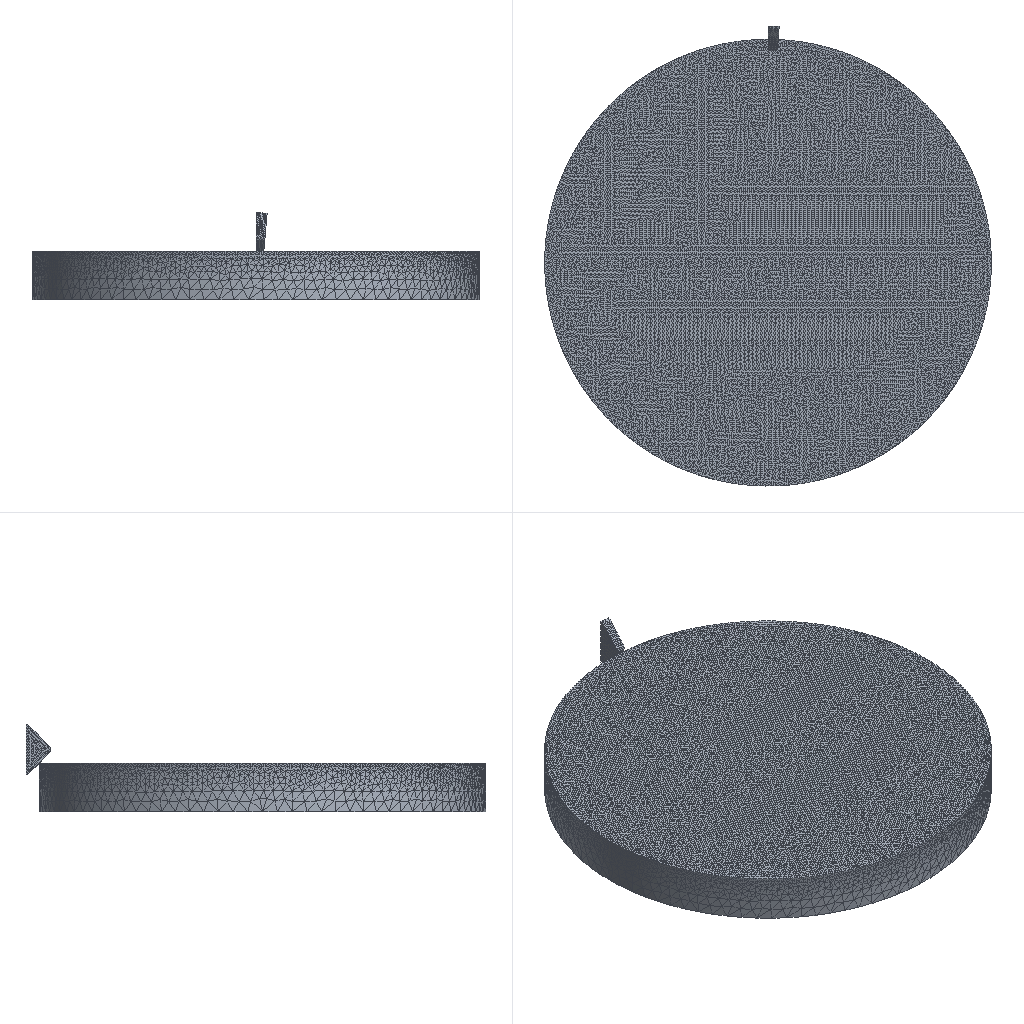Simulation study | abaqus
Set-up summary:
category,name,step,type,value,unit,region
solver,abaqus
solver,version,,,Abaqus/Explicit 3DEXPERIENCE R2017x
units,not stated in the deck,,not stated
analysis,deck,,dynamic temperature-displacement,dynamic temperature-displacement
load_step,Step-1,Step-1,dynamic temperature-displacement
load_step,requested,,,1
mesh,nodes,,,38093
mesh,elements,,,184281
element_type,C3D4T,,solid,184281
load,load commands in deck,,count,2
bc,support commands in deck,,count,15
material,STEEL304,,in results
material,YG,,in results
check,setup vs results,,match,"per instance, exact: element labels, types and connectivity; labels of the nodes the elements use; coordinates of those nodes at SINGLE_PRECISION in 2 of 2 instance(s)"
Abaqus input file, long lists of numbers shortened:
*Heading
** Job name: Job-1 Model name: Model-1
** Generated by: Abaqus/CAE 2017
*Preprint, echo=NO, model=NO, history=NO, contact=NO
**
** PARTS
**
*Part, name=tool_1
*Node
      1,   9.707,  0.2929,           0.
      2,           9.,           0.,           0.
** (493 more lines like these left out)
*Element, type=C3D4T
   1, 307, 308, 309, 310
   2, 311, 312, 313, 314
** (1925 more lines like these left out)
*Nset, nset=tool1, generate
   1,  495,    1
*Elset, elset=tool1, generate
    1,  1927,     1
*Nset, nset=T-TOOL, generate
   1,  495,    1
*Elset, elset=rigid, generate
    1,  1927,     1
*Elset, elset=_toolSurf_S1, internal
    6,   36,  397,  468,  496,  840,  861,  889,  901, 1128, 1170, 1358, 1372, 1427, 1478, 1497
 1511, 1537, 1538, 1557, 1595, 1596, 1637, 1638, 1655, 1682, 1684, 1700, 1703, 1715, 1720, 1725
** (1 more lines like these left out)
*Elset, elset=_toolSurf_S2, internal
   39,  280,  303,  518,  587,  593,  595,  701,  714, 1008, 1120, 1308, 1385, 1390, 1452, 1464
 1552, 1558, 1561, 1583, 1638, 1657, 1675, 1680, 1688, 1713, 1716, 1739, 1755, 1756, 1763, 1767
** (1 more lines like these left out)
*Elset, elset=_toolSurf_S3, internal
    4,   18,   22,   27,   38,   39,   51,   64,   76,   78,   80,   92,  100,  111,  113,  114
  115,  118,  137,  145,  149,  169,  188,  208,  212,  224,  263,  265,  266,  277,  280,  282
** (28 more lines like these left out)
*Elset, elset=_toolSurf_S4, internal
   36,  112,  125,  138,  190,  196,  202,  257,  277,  363,  376,  397,  469,  559,  562,  566
  594,  686,  785,  817,  901,  919,  960, 1078, 1170, 1309, 1336, 1359, 1421, 1425, 1502, 1546
** (2 more lines like these left out)
*Surface, type=ELEMENT, name=toolSurf
_toolSurf_S1, S1
_toolSurf_S2, S2
_toolSurf_S4, S4
_toolSurf_S3, S3
** Section: tool1
*Solid Section, elset=tool1, material=yg
,
*End Part
**
*Part, name=work
*Node
      1,          60.,           0.,          13.
      2,          60.,           0.,           0.
** (37596 more lines like these left out)
*Element, type=C3D4T
     1, 14286, 14287, 14288, 14289
     2, 14286, 14290, 14291, 14292
** (182352 more lines like these left out)
*Nset, nset=Set-1, generate
     1,  37598,      1
*Elset, elset=Set-1, generate
      1,  182354,       1
*Nset, nset=TWORK, generate
     1,  37598,      1
*Nset, nset=CHIP
     1,     3,     4,     5,     6,     7,     8,     9,    10,    11,    12,    13,    14,    15,    16,    17
    18,    19,    20,    21,    22,    23,    24,    25,    26,    27,    28,    29,    30,    31,    32,    33
** (1711 more lines like these left out)
** Section: work
*Solid Section, elset=Set-1, material=steel304
,
*End Part
**
**
** ASSEMBLY
**
*Assembly, name=Assembly
**
*Instance, name=tool_1, part=tool_1
42.307, 108.711, 111.816
42.307, 108.711, 111.816, 41.954, 107.858, 112.201, 94.132
*End Instance
**
*Instance, name=work, part=work
39.899, 52.214, 95.264
*End Instance
**
*Node
      1,   42.307,   115.782,    111.816
*Node
      2,    39.899,   52.214,   108.264
*Nset, nset=Set-8, instance=work
     2,   390,   391,   392,   393,   394,   395,   396,   397,   398,   399,   400,   401,   402,   403,   404
   405,   406,   407,   408,   409,   410,   411,   412,   413,   414,   415,   416,   417,   418,   419,   420
** (51 more lines like these left out)
*Elset, elset=Set-8, instance=work
    479,    734,    754,    773,    963,   1284,   1442,   1460,   1754,   1838,   1938,   2439,   2609,   3412,   3847,   5264
   6136,   6299,   6824,   7788,   8141,   9994,  10655,  11206,  11275,  12059,  12256,  12284,  12394,  12525,  12563,  12623
** (98 more lines like these left out)
*Nset, nset=rp1
 1,
*Nset, nset=rp2
 2,
*Nset, nset=work-yundong-yueshu, instance=work, generate
     1,  37598,      1
*Nset, nset=work-yundong-yueshu
 2,
*Elset, elset=work-yundong-yueshu, instance=work, generate
      1,  182354,       1
*Nset, nset=_PickedSet48, internal
 1,
*Elset, elset=_work-yundong_S3, internal, instance=work
    139,    148,    164,    183,    373,    479,    498,    509,    515,    530,    572,    573,    589,    599,    734,    749
    754,    773,    823,    867,    886,    934,    963,    974,   1034,   1180,   1284,   1288,   1442,   1460,   1462,   1465
** (1573 more lines like these left out)
*Elset, elset=_work-yundong_S4, internal, instance=work
    387,   1308,   1607,   1682,   1754,   2183,   2242,   2243,   2292,   2327,   2471,   2696,   2941,   5063,   5536,   5676
   5698,   8312,   9098,  10252,  10655,  12051,  12102,  12121,  12207,  12231,  12394,  12450,  12532,  12714,  12814,  12840
** (91 more lines like these left out)
*Elset, elset=_work-yundong_S2, internal, instance=work
    123,    399,   1518,   1659,   1938,   2067,   2315,   2393,   2507,   3847,   5086,   8799,   9659,  11511,  12089,  12172
  12210,  12275,  12359,  12503,  12563,  12745,  12753,  12783,  12856,  13201,  13287,  13707,  13758,  13884,  14035,  14171
** (68 more lines like these left out)
*Elset, elset=_work-yundong_S1, internal, instance=work
   1580,   6824,   7410,  11206,  12256,  12861,  13849,  14433,  14603,  14798,  15005,  15180,  15223,  15552,  15561,  15624
  16245,  16260,  16336,  16755,  16769,  16813,  17643,  17662,  17669,  17881,  17950,  17963,  18200,  19412,  19721,  19741
** (48 more lines like these left out)
*Surface, type=ELEMENT, name=work-yundong
_work-yundong_S3, S3
_work-yundong_S4, S4
_work-yundong_S2, S2
_work-yundong_S1, S1
*Surface, type=NODE, name=work_CHIP_CNS_, internal
work.CHIP, 1.
*Nset, nset="_T-work-Datum csys-1", internal
rp2,
*Transform, nset="_T-work-Datum csys-1"
          1.,           0.,           0.,           0.,           1.,           0.
** Constraint: Constraint-1
*Rigid Body, ref node=_PickedSet48, elset=tool_1.rigid
** Constraint: Constraint-2
*Coupling, constraint name=Constraint-2, ref node=rp2, surface=work-yundong
*Kinematic
*End Assembly
**
** MATERIALS
**
*Material, name=steel304
*Conductivity
 16.2,
*Damage Initiation, criterion=JOHNSON COOK
 0.0121,  0.4241, -0.6284,      0.,      0.,   1400.,     20.,    200.
*Damage Evolution, type=DISPLACEMENT
 0.1,
*Density
 7.9e-09,
*Elastic
193000., 0.29
*Expansion
 1.73e-05, 20.
 1.73e-05,100.
 1.78e-05,315.
 1.87e-05,650.
*Inelastic Heat Fraction
         0.9,
*Plastic, hardening=JOHNSON COOK
284.,  913., 0.609,  0.85, 1400.,   20.
*Rate Dependent, type=JOHNSON COOK
 0.1,200.
*Specific Heat
 5e+08,
*Material, name=yg
*Conductivity
110.,
*Density
 1.5e-08,
*Elastic
570000., 0.22
*Specific Heat
 2.03e+08,
**
** INTERACTION PROPERTIES
**
*Surface Interaction, name=IntProp-1
*Friction
 0.4,
*Surface Behavior, pressure-overclosure=HARD
*Gap Heat Generation
1., 0.5
**
** BOUNDARY CONDITIONS
**
** Name: BC-4 Type: 位移/转角
*Boundary
Set-8, 3, 3
Set-8, 4, 4
Set-8, 5, 5
**
** PREDEFINED FIELDS
**
** Name: Predefined Field-1   Type: Temperature
*Initial Conditions, type=TEMPERATURE
work.TWORK, 20.
** Name: Predefined Field-2   Type: Temperature
*Initial Conditions, type=TEMPERATURE
tool_1.T-TOOL, 20.
** ----------------------------------------------------------------
**
** STEP: Step-1
**
*Step, name=Step-1, nlgeom=YES
*Dynamic Temperature-displacement, Explicit
, 0.283
*Bulk Viscosity
0.06, 1.2
** Mass Scaling: Semi-Automatic
**               Whole Model
*Fixed Mass Scaling, factor=200.
**
** BOUNDARY CONDITIONS
**
** Name: BC-2 Type: 速度/角速度
*Boundary, type=VELOCITY
rp2, 1, 1
rp2, 2, 2
rp2, 3, 3
rp2, 4, 4
rp2, 5, 5
rp2, 6, 6, 22.2
** Name: BC-3 Type: 速度/角速度
*Boundary, type=VELOCITY
rp1, 1, 1
rp1, 2, 2, -1.06
rp1, 3, 3
rp1, 4, 4
rp1, 5, 5
rp1, 6, 6
**
** INTERACTIONS
**
** Interaction: Int-1
*Contact Pair, interaction=IntProp-1, mechanical constraint=KINEMATIC, cpset=Int-1
tool_1.toolSurf, work_CHIP_CNS_
**
** OUTPUT REQUESTS
**
*Restart, write, number interval=1, time marks=NO
**
** FIELD OUTPUT: F-Output-1
**
*Output, field
*Node Output
A, NT, RF, RFL, U, V
*Element Output, directions=YES
EVF, HFL, LE, PE, PEEQ, PEEQVAVG, PEVAVG, S, STATUS, SVAVG
*Contact Output
CSTRESS,
**
** HISTORY OUTPUT: H-Output-1
**
*Output, history, variable=PRESELECT
*End Step
Results summary:
result,step,Step-1,partial,increments=1 time=0.0/0.283
result,analysis,,,"dynamic temperature-displacement, explict"
result,last_loadstep,,,1
result,primary field,,,"U, NT11"
result,reaction total,,FX,601553.125,model units
result,reaction total,,FY,-690275.938,model units
result,reaction total,,FZ,0.0,model units